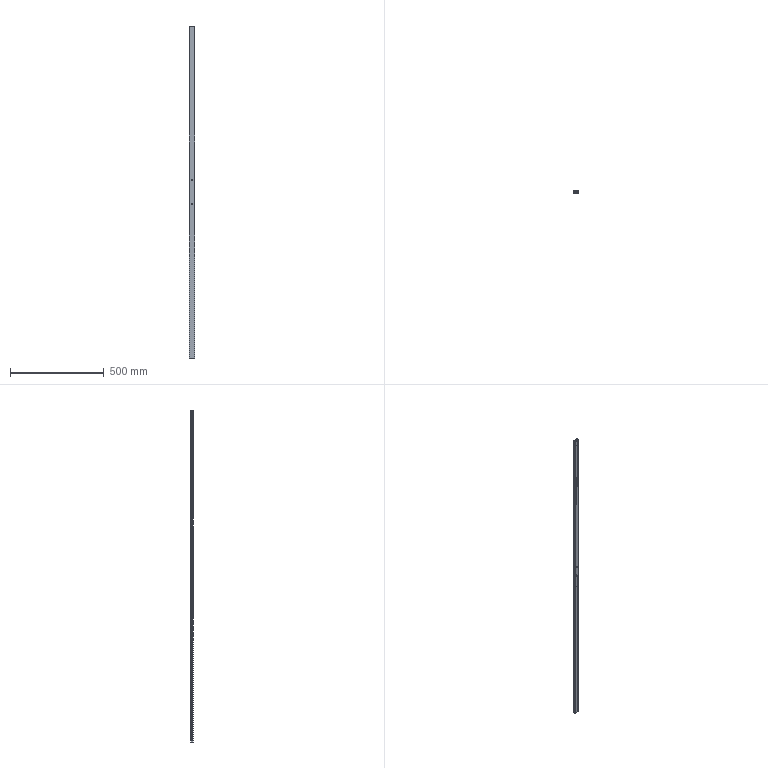Part | SolidWorks | features HoleWzd 3, BaseBody 1, MoveFace 1 | 1 solid | 176 faces | box 30 x 15 x 1772 mm | volume 426374 mm3 | cylinder 88 | plane 72 | cone 16 | commonest cylinder face diameters 5 x26 3.3 x24 4.5 x16 1 x12 2 x4 6.6 x4